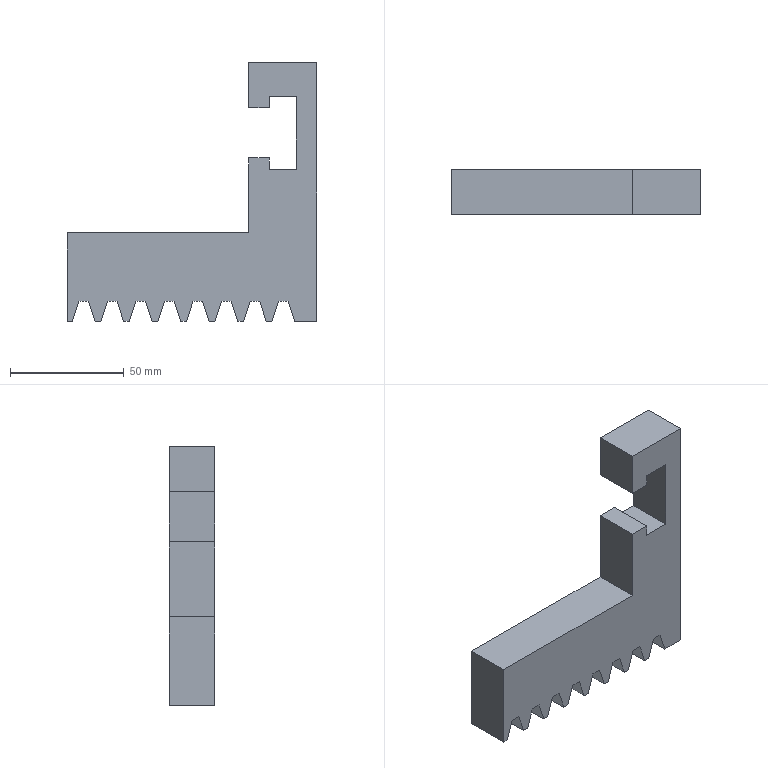Part | SolidWorks | features BaseBody 1 | 1 solid | 56 faces | box 110 x 20 x 114 mm | volume 108896 mm3 | plane 40 | cylinder 16 | commonest cylinder face diameters 94.224 x16